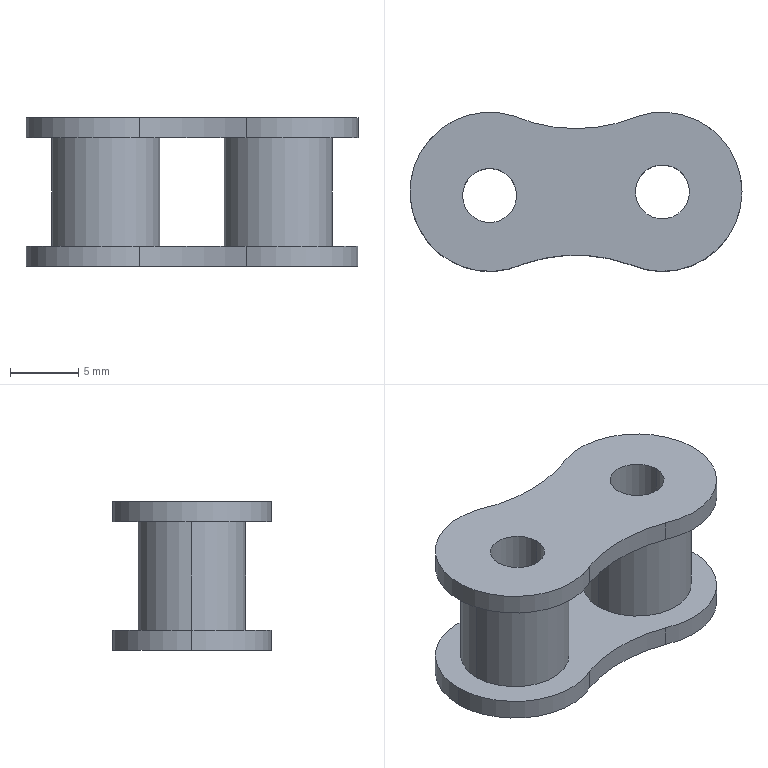Part | STEP file | CHEL40Achain-4 | 1 solid | 22 faces | box 24.4 x 11.7 x 10.95 mm | volume 1235 mm3 | cylinder 18 | plane 4 | commonest cylinder face diameters 11.7 x6 3.97 x4 7.95 x4 23.4 x4